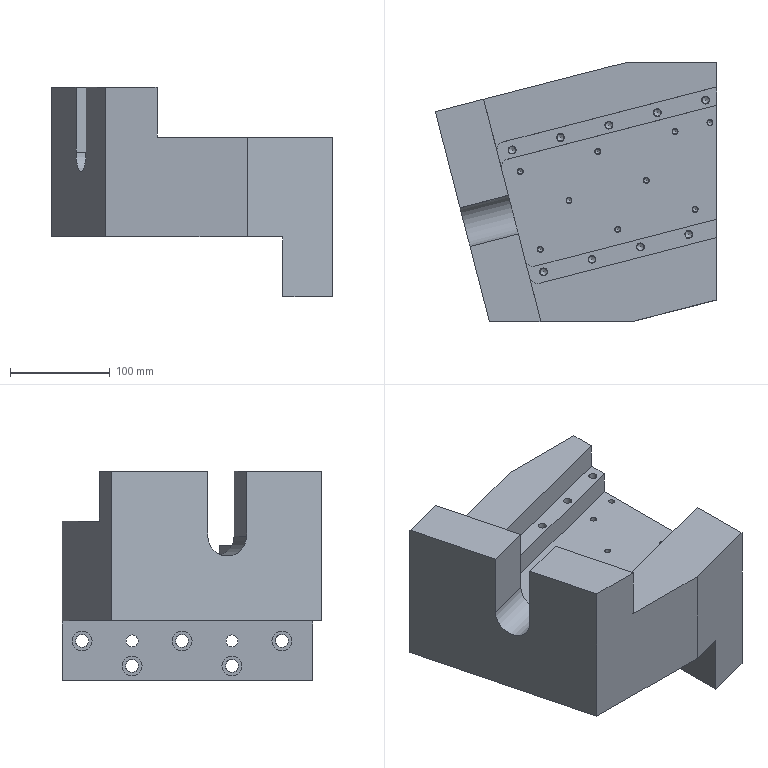Part | STEP file | 车灯-后视镜_id498_x_t | 1 solid | 117 faces | box 281.721 x 260 x 210 mm | volume 5973033 mm3 | cylinder 53 | plane 46 | cone 18 | commonest cylinder face diameters 5.1 x9 6 x9 6.9 x9 8 x9 13 x5 20 x5